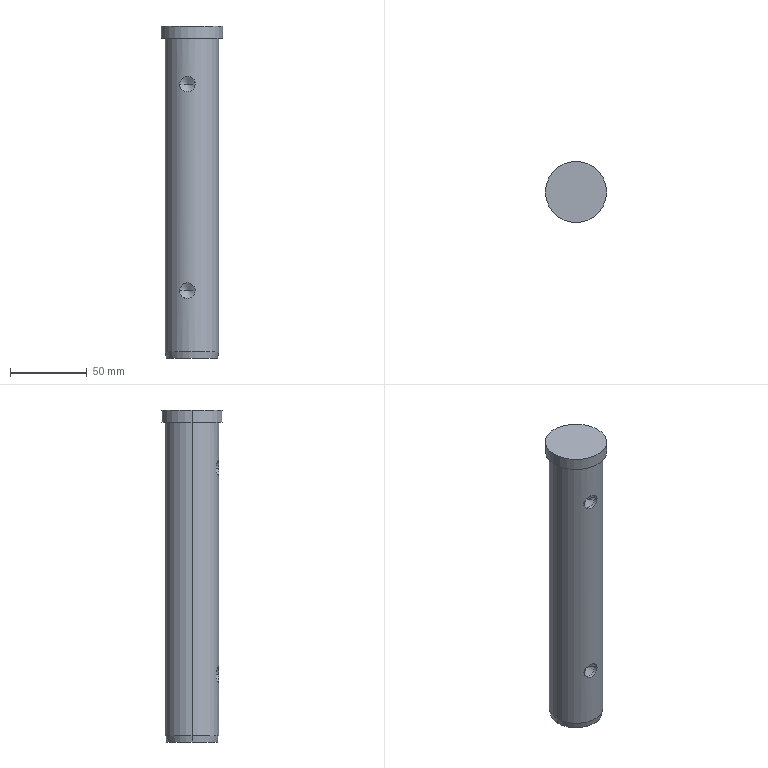Part | Creo | 1 solid | 17 faces | box 40 x 40 x 217 mm | volume 210497 mm3 | cylinder 8 | cone 6 | plane 3 | commonest cylinder face diameters 10.2 x4 35 x2 40 x2
STEP:
#1=CARTESIAN_POINT('',(0.,0.,0.));
#2=DIRECTION('',(0.,0.,1.));
#3=DIRECTION('',(1.,0.,0.));
#4=AXIS2_PLACEMENT_3D('',#1,#2,#3);
#5=CARTESIAN_POINT('',(-142.,-212.,112.5));
#6=VERTEX_POINT('',#5);
#7=CARTESIAN_POINT('',(-182.,-212.,112.5));
#8=VERTEX_POINT('',#7);
#9=CARTESIAN_POINT('',(-162.,-212.,112.5));
#10=DIRECTION('',(0.,0.,-1.));
#11=DIRECTION('',(1.,0.,0.));
#12=AXIS2_PLACEMENT_3D('',#9,#10,#11);
#13=CIRCLE('',#12,20.);
#14=EDGE_CURVE('',#6,#8,#13,.T.);
#15=ORIENTED_EDGE('',*,*,#14,.T.);
#16=CARTESIAN_POINT('',(-182.,-212.,120.5));
#17=VERTEX_POINT('',#16);
#18=CARTESIAN_POINT('',(-182.,-212.,112.5));
#19=DIRECTION('',(0.,0.,1.));
#20=VECTOR('',#19,8.);
#21=LINE('',#18,#20);
#22=EDGE_CURVE('',#8,#17,#21,.T.);
#23=ORIENTED_EDGE('',*,*,#22,.T.);
#24=CARTESIAN_POINT('',(-142.,-212.,120.5));
#25=VERTEX_POINT('',#24);
#26=CARTESIAN_POINT('',(-162.,-212.,120.5));
#27=DIRECTION('',(0.,0.,1.));
#28=DIRECTION('',(-1.,0.,0.));
#29=AXIS2_PLACEMENT_3D('',#26,#27,#28);
#30=CIRCLE('',#29,20.);
#31=EDGE_CURVE('',#17,#25,#30,.T.);
#32=ORIENTED_EDGE('',*,*,#31,.T.);
#33=CARTESIAN_POINT('',(-142.,-212.,112.5));
#34=DIRECTION('',(0.,0.,1.));
#35=VECTOR('',#34,8.);
#36=LINE('',#33,#35);
#37=EDGE_CURVE('',#6,#25,#36,.T.);
#38=ORIENTED_EDGE('',*,*,#37,.F.);
#39=EDGE_LOOP('',(#15,#23,#32,#38));
#40=FACE_OUTER_BOUND('',#39,.F.);
#41=CARTESIAN_POINT('',(-162.,-212.,112.5));
#42=DIRECTION('',(0.,0.,1.));
#43=DIRECTION('',(-1.,0.,0.));
#44=AXIS2_PLACEMENT_3D('',#41,#42,#43);
#45=CYLINDRICAL_SURFACE('',#44,20.);
#46=ADVANCED_FACE('',(#40),#45,.T.);
#47=ORIENTED_EDGE('',*,*,#14,.F.);
#48=CARTESIAN_POINT('',(-162.,-212.,112.5));
#49=DIRECTION('',(0.,0.,-1.));
#50=DIRECTION('',(-1.,0.,0.));
#51=AXIS2_PLACEMENT_3D('',#48,#49,#50);
#52=CIRCLE('',#51,20.);
#53=EDGE_CURVE('',#8,#6,#52,.T.);
#54=ORIENTED_EDGE('',*,*,#53,.F.);
#55=EDGE_LOOP('',(#47,#54));
#56=FACE_OUTER_BOUND('',#55,.F.);
#57=CARTESIAN_POINT('',(-179.5,-212.,112.5));
#58=VERTEX_POINT('',#57);
#59=CARTESIAN_POINT('',(-144.5,-212.,112.5));
#60=VERTEX_POINT('',#59);
#61=CARTESIAN_POINT('',(-162.,-212.,112.5));
#62=DIRECTION('',(0.,0.,1.));
#63=DIRECTION('',(-1.,0.,0.));
#64=AXIS2_PLACEMENT_3D('',#61,#62,#63);
#65=CIRCLE('',#64,17.5);
#66=EDGE_CURVE('',#58,#60,#65,.T.);
#67=ORIENTED_EDGE('',*,*,#66,.F.);
#68=CARTESIAN_POINT('',(-162.,-212.,112.5));
#69=DIRECTION('',(0.,0.,1.));
#70=DIRECTION('',(1.,0.,0.));
#71=AXIS2_PLACEMENT_3D('',#68,#69,#70);
#72=CIRCLE('',#71,17.5);
#73=EDGE_CURVE('',#60,#58,#72,.T.);
#74=ORIENTED_EDGE('',*,*,#73,.F.);
#75=EDGE_LOOP('',(#67,#74));
#76=FACE_BOUND('',#75,.F.);
#77=CARTESIAN_POINT('',(-162.,-212.,112.5));
#78=DIRECTION('',(0.,0.,1.));
#79=DIRECTION('',(-1.,0.,0.));
#80=AXIS2_PLACEMENT_3D('',#77,#78,#79);
#81=PLANE('',#80);
#82=ADVANCED_FACE('',(#56,#76),#81,.F.);
#83=CARTESIAN_POINT('',(-144.5,-212.,-92.5));
#84=VERTEX_POINT('',#83);
#85=CARTESIAN_POINT('',(-179.5,-212.,-92.5));
#86=VERTEX_POINT('',#85);
#87=CARTESIAN_POINT('',(-162.,-212.,-92.5));
#88=DIRECTION('',(0.,0.,-1.));
#89=DIRECTION('',(1.,0.,0.));
#90=AXIS2_PLACEMENT_3D('',#87,#88,#89);
#91=CIRCLE('',#90,17.5);
#92=EDGE_CURVE('',#84,#86,#91,.T.);
#93=ORIENTED_EDGE('',*,*,#92,.T.);
#94=CARTESIAN_POINT('',(-179.5,-212.,112.5));
#95=DIRECTION('',(0.,0.,-1.));
#96=VECTOR('',#95,205.);
#97=LINE('',#94,#96);
#98=EDGE_CURVE('',#58,#86,#97,.T.);
#99=ORIENTED_EDGE('',*,*,#98,.F.);
#100=ORIENTED_EDGE('',*,*,#66,.T.);
#101=CARTESIAN_POINT('',(-144.5,-212.,112.5));
#102=DIRECTION('',(0.,0.,-1.));
#103=VECTOR('',#102,205.);
#104=LINE('',#101,#103);
#105=EDGE_CURVE('',#60,#84,#104,.T.);
#106=ORIENTED_EDGE('',*,*,#105,.T.);
#107=EDGE_LOOP('',(#93,#99,#100,#106));
#108=FACE_OUTER_BOUND('',#107,.F.);
#109=CARTESIAN_POINT('',(-170.1,-227.513,82.5));
#110=VERTEX_POINT('',#109);
#111=CARTESIAN_POINT('',(-159.9,-229.374,82.5));
#112=VERTEX_POINT('',#111);
#113=CARTESIAN_POINT('',(-170.1,-227.513,82.5));
#114=CARTESIAN_POINT('',(-170.1,-227.513,82.927));
#115=CARTESIAN_POINT('',(-169.996,-227.567,83.761));
#116=CARTESIAN_POINT('',(-169.521,-227.806,84.981));
#117=CARTESIAN_POINT('',(-168.726,-228.167,86.072));
#118=CARTESIAN_POINT('',(-167.635,-228.584,86.939));
#119=CARTESIAN_POINT('',(-166.374,-228.962,87.472));
#120=CARTESIAN_POINT('',(-165.054,-229.249,87.656));
#121=CARTESIAN_POINT('',(-163.737,-229.43,87.501));
#122=CARTESIAN_POINT('',(-162.478,-229.507,87.001));
#123=CARTESIAN_POINT('',(-161.392,-229.498,86.189));
#124=CARTESIAN_POINT('',(-160.545,-229.444,85.108));
#125=CARTESIAN_POINT('',(-160.015,-229.388,83.829));
#126=CARTESIAN_POINT('',(-159.9,-229.374,82.953));
#127=CARTESIAN_POINT('',(-159.9,-229.374,82.5));
#128=B_SPLINE_CURVE_WITH_KNOTS('',3,(#113,#114,#115,#116,#117,#118,#119,#120,#121,#122,#123,#124,#125,#126,#127),.UNSPECIFIED.,.F.,.F.,(4,1,1,1,1,1,1,1,1,1,1,1,4),(0.,0.08333,0.1667,0.25,0.3333,0.4167,0.5,0.5833,0.6667,0.75,0.8333,0.9167,1.),.UNSPECIFIED.);
#129=EDGE_CURVE('',#110,#112,#128,.T.);
#130=ORIENTED_EDGE('',*,*,#129,.F.);
#131=CARTESIAN_POINT('',(-159.9,-229.374,82.5));
#132=CARTESIAN_POINT('',(-159.9,-229.374,82.038));
#133=CARTESIAN_POINT('',(-160.02,-229.389,81.149));
#134=CARTESIAN_POINT('',(-160.556,-229.445,79.875));
#135=CARTESIAN_POINT('',(-161.399,-229.499,78.805));
#136=CARTESIAN_POINT('',(-162.485,-229.507,77.995));
#137=CARTESIAN_POINT('',(-163.748,-229.429,77.496));
#138=CARTESIAN_POINT('',(-165.067,-229.247,77.344));
#139=CARTESIAN_POINT('',(-166.382,-228.96,77.53));
#140=CARTESIAN_POINT('',(-167.638,-228.583,78.063));
#141=CARTESIAN_POINT('',(-168.727,-228.166,78.93));
#142=CARTESIAN_POINT('',(-169.523,-227.805,80.022));
#143=CARTESIAN_POINT('',(-169.996,-227.567,81.241));
#144=CARTESIAN_POINT('',(-170.1,-227.513,82.073));
#145=CARTESIAN_POINT('',(-170.1,-227.513,82.5));
#146=B_SPLINE_CURVE_WITH_KNOTS('',3,(#131,#132,#133,#134,#135,#136,#137,#138,#139,#140,#141,#142,#143,#144,#145),.UNSPECIFIED.,.F.,.F.,(4,1,1,1,1,1,1,1,1,1,1,1,4),(0.,0.08333,0.1667,0.25,0.3333,0.4167,0.5,0.5833,0.6667,0.75,0.8333,0.9167,1.),.UNSPECIFIED.);
#147=EDGE_CURVE('',#112,#110,#146,.T.);
#148=ORIENTED_EDGE('',*,*,#147,.F.);
#149=EDGE_LOOP('',(#130,#148));
#150=FACE_BOUND('',#149,.F.);
#151=CARTESIAN_POINT('',(-170.1,-227.513,-52.5));
#152=VERTEX_POINT('',#151);
#153=CARTESIAN_POINT('',(-159.9,-229.374,-52.5));
#154=VERTEX_POINT('',#153);
#155=CARTESIAN_POINT('',(-170.1,-227.513,-52.5));
#156=CARTESIAN_POINT('',(-170.1,-227.513,-52.073));
#157=CARTESIAN_POINT('',(-169.996,-227.567,-51.239));
#158=CARTESIAN_POINT('',(-169.521,-227.806,-50.019));
#159=CARTESIAN_POINT('',(-168.726,-228.167,-48.928));
#160=CARTESIAN_POINT('',(-167.635,-228.584,-48.061));
#161=CARTESIAN_POINT('',(-166.374,-228.962,-47.528));
#162=CARTESIAN_POINT('',(-165.054,-229.249,-47.344));
#163=CARTESIAN_POINT('',(-163.737,-229.43,-47.499));
#164=CARTESIAN_POINT('',(-162.478,-229.507,-47.999));
#165=CARTESIAN_POINT('',(-161.392,-229.498,-48.811));
#166=CARTESIAN_POINT('',(-160.545,-229.444,-49.892));
#167=CARTESIAN_POINT('',(-160.015,-229.388,-51.171));
#168=CARTESIAN_POINT('',(-159.9,-229.374,-52.047));
#169=CARTESIAN_POINT('',(-159.9,-229.374,-52.5));
#170=B_SPLINE_CURVE_WITH_KNOTS('',3,(#155,#156,#157,#158,#159,#160,#161,#162,#163,#164,#165,#166,#167,#168,#169),.UNSPECIFIED.,.F.,.F.,(4,1,1,1,1,1,1,1,1,1,1,1,4),(0.,0.08333,0.1667,0.25,0.3333,0.4167,0.5,0.5833,0.6667,0.75,0.8333,0.9167,1.),.UNSPECIFIED.);
#171=EDGE_CURVE('',#152,#154,#170,.T.);
#172=ORIENTED_EDGE('',*,*,#171,.F.);
#173=CARTESIAN_POINT('',(-159.9,-229.374,-52.5));
#174=CARTESIAN_POINT('',(-159.9,-229.374,-52.962));
#175=CARTESIAN_POINT('',(-160.02,-229.389,-53.851));
#176=CARTESIAN_POINT('',(-160.556,-229.445,-55.125));
#177=CARTESIAN_POINT('',(-161.399,-229.499,-56.195));
#178=CARTESIAN_POINT('',(-162.485,-229.507,-57.005));
#179=CARTESIAN_POINT('',(-163.748,-229.429,-57.504));
#180=CARTESIAN_POINT('',(-165.067,-229.247,-57.656));
#181=CARTESIAN_POINT('',(-166.382,-228.96,-57.47));
#182=CARTESIAN_POINT('',(-167.638,-228.583,-56.937));
#183=CARTESIAN_POINT('',(-168.727,-228.166,-56.07));
#184=CARTESIAN_POINT('',(-169.523,-227.805,-54.978));
#185=CARTESIAN_POINT('',(-169.996,-227.567,-53.759));
#186=CARTESIAN_POINT('',(-170.1,-227.513,-52.927));
#187=CARTESIAN_POINT('',(-170.1,-227.513,-52.5));
#188=B_SPLINE_CURVE_WITH_KNOTS('',3,(#173,#174,#175,#176,#177,#178,#179,#180,#181,#182,#183,#184,#185,#186,#187),.UNSPECIFIED.,.F.,.F.,(4,1,1,1,1,1,1,1,1,1,1,1,4),(0.,0.08333,0.1667,0.25,0.3333,0.4167,0.5,0.5833,0.6667,0.75,0.8333,0.9167,1.),.UNSPECIFIED.);
#189=EDGE_CURVE('',#154,#152,#188,.T.);
#190=ORIENTED_EDGE('',*,*,#189,.F.);
#191=EDGE_LOOP('',(#172,#190));
#192=FACE_BOUND('',#191,.F.);
#193=CARTESIAN_POINT('',(-162.,-212.,112.5));
#194=DIRECTION('',(0.,0.,-1.));
#195=DIRECTION('',(1.,0.,0.));
#196=AXIS2_PLACEMENT_3D('',#193,#194,#195);
#197=CYLINDRICAL_SURFACE('',#196,17.5);
#198=ADVANCED_FACE('',(#108,#150,#192),#197,.T.);
#199=ORIENTED_EDGE('',*,*,#171,.T.);
#200=CARTESIAN_POINT('',(-159.9,-227.1,-52.5));
#201=VERTEX_POINT('',#200);
#202=CARTESIAN_POINT('',(-159.9,-227.1,-52.5));
#203=DIRECTION('',(-0.000000022,-1.,-0.0001831));
#204=VECTOR('',#203,2.274);
#205=LINE('',#202,#204);
#206=EDGE_CURVE('',#201,#154,#205,.T.);
#207=ORIENTED_EDGE('',*,*,#206,.F.);
#208=CARTESIAN_POINT('',(-170.1,-227.1,-52.5));
#209=VERTEX_POINT('',#208);
#210=CARTESIAN_POINT('',(-165.,-227.1,-52.5));
#211=DIRECTION('',(0.,-1.,0.));
#212=DIRECTION('',(1.,0.,0.));
#213=AXIS2_PLACEMENT_3D('',#210,#211,#212);
#214=CIRCLE('',#213,5.1);
#215=EDGE_CURVE('',#201,#209,#214,.T.);
#216=ORIENTED_EDGE('',*,*,#215,.T.);
#217=CARTESIAN_POINT('',(-170.1,-227.1,-52.5));
#218=DIRECTION('',(0.,-1.,0.));
#219=VECTOR('',#218,0.4126);
#220=LINE('',#217,#219);
#221=EDGE_CURVE('',#209,#152,#220,.T.);
#222=ORIENTED_EDGE('',*,*,#221,.T.);
#223=EDGE_LOOP('',(#199,#207,#216,#222));
#224=FACE_OUTER_BOUND('',#223,.F.);
#225=CARTESIAN_POINT('',(-165.,-300.,-52.5));
#226=DIRECTION('',(0.,-1.,0.));
#227=DIRECTION('',(-1.,0.,0.));
#228=AXIS2_PLACEMENT_3D('',#225,#226,#227);
#229=CYLINDRICAL_SURFACE('',#228,5.1);
#230=ADVANCED_FACE('',(#224),#229,.F.);
#231=ORIENTED_EDGE('',*,*,#189,.T.);
#232=ORIENTED_EDGE('',*,*,#221,.F.);
#233=CARTESIAN_POINT('',(-165.,-227.1,-52.5));
#234=DIRECTION('',(0.,-1.,0.));
#235=DIRECTION('',(-1.,0.,0.));
#236=AXIS2_PLACEMENT_3D('',#233,#234,#235);
#237=CIRCLE('',#236,5.1);
#238=EDGE_CURVE('',#209,#201,#237,.T.);
#239=ORIENTED_EDGE('',*,*,#238,.T.);
#240=ORIENTED_EDGE('',*,*,#206,.T.);
#241=EDGE_LOOP('',(#231,#232,#239,#240));
#242=FACE_OUTER_BOUND('',#241,.F.);
#243=CARTESIAN_POINT('',(-165.,-300.,-52.5));
#244=DIRECTION('',(0.,-1.,0.));
#245=DIRECTION('',(-1.,0.,0.));
#246=AXIS2_PLACEMENT_3D('',#243,#244,#245);
#247=CYLINDRICAL_SURFACE('',#246,5.1);
#248=ADVANCED_FACE('',(#242),#247,.F.);
#249=ORIENTED_EDGE('',*,*,#238,.F.);
#250=CARTESIAN_POINT('',(-165.,-224.036,-52.5));
#251=VERTEX_POINT('',#250);
#252=CARTESIAN_POINT('',(-165.,-224.036,-52.5));
#253=DIRECTION('',(-0.8572,-0.515,0.));
#254=VECTOR('',#253,5.95);
#255=LINE('',#252,#254);
#256=EDGE_CURVE('',#251,#209,#255,.T.);
#257=ORIENTED_EDGE('',*,*,#256,.F.);
#258=CARTESIAN_POINT('',(-165.,-224.036,-52.5));
#259=DIRECTION('',(0.8572,-0.515,0.));
#260=VECTOR('',#259,5.95);
#261=LINE('',#258,#260);
#262=EDGE_CURVE('',#251,#201,#261,.T.);
#263=ORIENTED_EDGE('',*,*,#262,.T.);
#264=EDGE_LOOP('',(#249,#257,#263));
#265=FACE_OUTER_BOUND('',#264,.F.);
#266=CARTESIAN_POINT('',(-165.,-225.637,-52.5));
#267=DIRECTION('',(0.,-1.,0.));
#268=DIRECTION('',(-1.,0.,0.));
#269=AXIS2_PLACEMENT_3D('',#266,#267,#268);
#270=CONICAL_SURFACE('',#269,2.665,59.);
#271=ADVANCED_FACE('',(#265),#270,.F.);
#272=ORIENTED_EDGE('',*,*,#215,.F.);
#273=ORIENTED_EDGE('',*,*,#262,.F.);
#274=ORIENTED_EDGE('',*,*,#256,.T.);
#275=EDGE_LOOP('',(#272,#273,#274));
#276=FACE_OUTER_BOUND('',#275,.F.);
#277=CARTESIAN_POINT('',(-165.,-225.637,-52.5));
#278=DIRECTION('',(0.,-1.,0.));
#279=DIRECTION('',(-1.,0.,0.));
#280=AXIS2_PLACEMENT_3D('',#277,#278,#279);
#281=CONICAL_SURFACE('',#280,2.665,59.);
#282=ADVANCED_FACE('',(#276),#281,.F.);
#283=ORIENTED_EDGE('',*,*,#129,.T.);
#284=CARTESIAN_POINT('',(-159.9,-227.1,82.5));
#285=VERTEX_POINT('',#284);
#286=CARTESIAN_POINT('',(-159.9,-227.1,82.5));
#287=DIRECTION('',(-0.000000022,-1.,-0.0001831));
#288=VECTOR('',#287,2.274);
#289=LINE('',#286,#288);
#290=EDGE_CURVE('',#285,#112,#289,.T.);
#291=ORIENTED_EDGE('',*,*,#290,.F.);
#292=CARTESIAN_POINT('',(-170.1,-227.1,82.5));
#293=VERTEX_POINT('',#292);
#294=CARTESIAN_POINT('',(-165.,-227.1,82.5));
#295=DIRECTION('',(0.,-1.,0.));
#296=DIRECTION('',(1.,0.,0.));
#297=AXIS2_PLACEMENT_3D('',#294,#295,#296);
#298=CIRCLE('',#297,5.1);
#299=EDGE_CURVE('',#285,#293,#298,.T.);
#300=ORIENTED_EDGE('',*,*,#299,.T.);
#301=CARTESIAN_POINT('',(-170.1,-227.1,82.5));
#302=DIRECTION('',(0.,-1.,0.));
#303=VECTOR('',#302,0.4126);
#304=LINE('',#301,#303);
#305=EDGE_CURVE('',#293,#110,#304,.T.);
#306=ORIENTED_EDGE('',*,*,#305,.T.);
#307=EDGE_LOOP('',(#283,#291,#300,#306));
#308=FACE_OUTER_BOUND('',#307,.F.);
#309=CARTESIAN_POINT('',(-165.,-300.,82.5));
#310=DIRECTION('',(0.,-1.,0.));
#311=DIRECTION('',(-1.,0.,0.));
#312=AXIS2_PLACEMENT_3D('',#309,#310,#311);
#313=CYLINDRICAL_SURFACE('',#312,5.1);
#314=ADVANCED_FACE('',(#308),#313,.F.);
#315=ORIENTED_EDGE('',*,*,#147,.T.);
#316=ORIENTED_EDGE('',*,*,#305,.F.);
#317=CARTESIAN_POINT('',(-165.,-227.1,82.5));
#318=DIRECTION('',(0.,-1.,0.));
#319=DIRECTION('',(-1.,0.,0.));
#320=AXIS2_PLACEMENT_3D('',#317,#318,#319);
#321=CIRCLE('',#320,5.1);
#322=EDGE_CURVE('',#293,#285,#321,.T.);
#323=ORIENTED_EDGE('',*,*,#322,.T.);
#324=ORIENTED_EDGE('',*,*,#290,.T.);
#325=EDGE_LOOP('',(#315,#316,#323,#324));
#326=FACE_OUTER_BOUND('',#325,.F.);
#327=CARTESIAN_POINT('',(-165.,-300.,82.5));
#328=DIRECTION('',(0.,-1.,0.));
#329=DIRECTION('',(-1.,0.,0.));
#330=AXIS2_PLACEMENT_3D('',#327,#328,#329);
#331=CYLINDRICAL_SURFACE('',#330,5.1);
#332=ADVANCED_FACE('',(#326),#331,.F.);
#333=ORIENTED_EDGE('',*,*,#322,.F.);
#334=CARTESIAN_POINT('',(-165.,-224.036,82.5));
#335=VERTEX_POINT('',#334);
#336=CARTESIAN_POINT('',(-165.,-224.036,82.5));
#337=DIRECTION('',(-0.8572,-0.515,0.));
#338=VECTOR('',#337,5.95);
#339=LINE('',#336,#338);
#340=EDGE_CURVE('',#335,#293,#339,.T.);
#341=ORIENTED_EDGE('',*,*,#340,.F.);
#342=CARTESIAN_POINT('',(-165.,-224.036,82.5));
#343=DIRECTION('',(0.8572,-0.515,0.));
#344=VECTOR('',#343,5.95);
#345=LINE('',#342,#344);
#346=EDGE_CURVE('',#335,#285,#345,.T.);
#347=ORIENTED_EDGE('',*,*,#346,.T.);
#348=EDGE_LOOP('',(#333,#341,#347));
#349=FACE_OUTER_BOUND('',#348,.F.);
#350=CARTESIAN_POINT('',(-165.,-225.637,82.5));
#351=DIRECTION('',(0.,-1.,0.));
#352=DIRECTION('',(-1.,0.,0.));
#353=AXIS2_PLACEMENT_3D('',#350,#351,#352);
#354=CONICAL_SURFACE('',#353,2.665,59.);
#355=ADVANCED_FACE('',(#349),#354,.F.);
#356=ORIENTED_EDGE('',*,*,#299,.F.);
#357=ORIENTED_EDGE('',*,*,#346,.F.);
#358=ORIENTED_EDGE('',*,*,#340,.T.);
#359=EDGE_LOOP('',(#356,#357,#358));
#360=FACE_OUTER_BOUND('',#359,.F.);
#361=CARTESIAN_POINT('',(-165.,-225.637,82.5));
#362=DIRECTION('',(0.,-1.,0.));
#363=DIRECTION('',(-1.,0.,0.));
#364=AXIS2_PLACEMENT_3D('',#361,#362,#363);
#365=CONICAL_SURFACE('',#364,2.665,59.);
#366=ADVANCED_FACE('',(#360),#365,.F.);
#367=ORIENTED_EDGE('',*,*,#92,.F.);
#368=CARTESIAN_POINT('',(-145.205,-212.,-96.5));
#369=VERTEX_POINT('',#368);
#370=CARTESIAN_POINT('',(-145.205,-212.,-96.5));
#371=DIRECTION('',(0.1736,0.,0.9848));
#372=VECTOR('',#371,4.062);
#373=LINE('',#370,#372);
#374=EDGE_CURVE('',#369,#84,#373,.T.);
#375=ORIENTED_EDGE('',*,*,#374,.F.);
#376=CARTESIAN_POINT('',(-178.795,-212.,-96.5));
#377=VERTEX_POINT('',#376);
#378=CARTESIAN_POINT('',(-162.,-212.,-96.5));
#379=DIRECTION('',(0.,0.,-1.));
#380=DIRECTION('',(1.,0.,0.));
#381=AXIS2_PLACEMENT_3D('',#378,#379,#380);
#382=CIRCLE('',#381,16.795);
#383=EDGE_CURVE('',#369,#377,#382,.T.);
#384=ORIENTED_EDGE('',*,*,#383,.T.);
#385=CARTESIAN_POINT('',(-178.795,-212.,-96.5));
#386=DIRECTION('',(-0.1736,0.,0.9848));
#387=VECTOR('',#386,4.062);
#388=LINE('',#385,#387);
#389=EDGE_CURVE('',#377,#86,#388,.T.);
#390=ORIENTED_EDGE('',*,*,#389,.T.);
#391=EDGE_LOOP('',(#367,#375,#384,#390));
#392=FACE_OUTER_BOUND('',#391,.F.);
#393=CARTESIAN_POINT('',(-162.,-212.,-94.5));
#394=DIRECTION('',(0.,0.,1.));
#395=DIRECTION('',(-1.,0.,0.));
#396=AXIS2_PLACEMENT_3D('',#393,#394,#395);
#397=CONICAL_SURFACE('',#396,17.147,10.);
#398=ADVANCED_FACE('',(#392),#397,.T.);
#399=CARTESIAN_POINT('',(-162.,-212.,-92.5));
#400=DIRECTION('',(0.,0.,-1.));
#401=DIRECTION('',(-1.,0.,0.));
#402=AXIS2_PLACEMENT_3D('',#399,#400,#401);
#403=CIRCLE('',#402,17.5);
#404=EDGE_CURVE('',#86,#84,#403,.T.);
#405=ORIENTED_EDGE('',*,*,#404,.F.);
#406=ORIENTED_EDGE('',*,*,#389,.F.);
#407=CARTESIAN_POINT('',(-162.,-212.,-96.5));
#408=DIRECTION('',(0.,0.,-1.));
#409=DIRECTION('',(-1.,0.,0.));
#410=AXIS2_PLACEMENT_3D('',#407,#408,#409);
#411=CIRCLE('',#410,16.795);
#412=EDGE_CURVE('',#377,#369,#411,.T.);
#413=ORIENTED_EDGE('',*,*,#412,.T.);
#414=ORIENTED_EDGE('',*,*,#374,.T.);
#415=EDGE_LOOP('',(#405,#406,#413,#414));
#416=FACE_OUTER_BOUND('',#415,.F.);
#417=CARTESIAN_POINT('',(-162.,-212.,-94.5));
#418=DIRECTION('',(0.,0.,1.));
#419=DIRECTION('',(-1.,0.,0.));
#420=AXIS2_PLACEMENT_3D('',#417,#418,#419);
#421=CONICAL_SURFACE('',#420,17.147,10.);
#422=ADVANCED_FACE('',(#416),#421,.T.);
#423=ORIENTED_EDGE('',*,*,#404,.T.);
#424=ORIENTED_EDGE('',*,*,#105,.F.);
#425=ORIENTED_EDGE('',*,*,#73,.T.);
#426=ORIENTED_EDGE('',*,*,#98,.T.);
#427=EDGE_LOOP('',(#423,#424,#425,#426));
#428=FACE_OUTER_BOUND('',#427,.F.);
#429=CARTESIAN_POINT('',(-162.,-212.,112.5));
#430=DIRECTION('',(0.,0.,-1.));
#431=DIRECTION('',(1.,0.,0.));
#432=AXIS2_PLACEMENT_3D('',#429,#430,#431);
#433=CYLINDRICAL_SURFACE('',#432,17.5);
#434=ADVANCED_FACE('',(#428),#433,.T.);
#435=ORIENTED_EDGE('',*,*,#412,.F.);
#436=ORIENTED_EDGE('',*,*,#383,.F.);
#437=EDGE_LOOP('',(#435,#436));
#438=FACE_OUTER_BOUND('',#437,.F.);
#439=CARTESIAN_POINT('',(-162.,-212.,-96.5));
#440=DIRECTION('',(0.,0.,-1.));
#441=DIRECTION('',(1.,0.,0.));
#442=AXIS2_PLACEMENT_3D('',#439,#440,#441);
#443=PLANE('',#442);
#444=ADVANCED_FACE('',(#438),#443,.T.);
#445=ORIENTED_EDGE('',*,*,#53,.T.);
#446=ORIENTED_EDGE('',*,*,#37,.T.);
#447=CARTESIAN_POINT('',(-162.,-212.,120.5));
#448=DIRECTION('',(0.,0.,1.));
#449=DIRECTION('',(1.,0.,0.));
#450=AXIS2_PLACEMENT_3D('',#447,#448,#449);
#451=CIRCLE('',#450,20.);
#452=EDGE_CURVE('',#25,#17,#451,.T.);
#453=ORIENTED_EDGE('',*,*,#452,.T.);
#454=ORIENTED_EDGE('',*,*,#22,.F.);
#455=EDGE_LOOP('',(#445,#446,#453,#454));
#456=FACE_OUTER_BOUND('',#455,.F.);
#457=CARTESIAN_POINT('',(-162.,-212.,112.5));
#458=DIRECTION('',(0.,0.,1.));
#459=DIRECTION('',(-1.,0.,0.));
#460=AXIS2_PLACEMENT_3D('',#457,#458,#459);
#461=CYLINDRICAL_SURFACE('',#460,20.);
#462=ADVANCED_FACE('',(#456),#461,.T.);
#463=ORIENTED_EDGE('',*,*,#452,.F.);
#464=ORIENTED_EDGE('',*,*,#31,.F.);
#465=EDGE_LOOP('',(#463,#464));
#466=FACE_OUTER_BOUND('',#465,.F.);
#467=CARTESIAN_POINT('',(-162.,-212.,120.5));
#468=DIRECTION('',(0.,0.,1.));
#469=DIRECTION('',(-1.,0.,0.));
#470=AXIS2_PLACEMENT_3D('',#467,#468,#469);
#471=PLANE('',#470);
#472=ADVANCED_FACE('',(#466),#471,.T.);
#473=CLOSED_SHELL('',(#46,#82,#198,#230,#248,#271,#282,#314,#332,#355,#366,#398,#422,#434,#444,#462,#472));
#474=MANIFOLD_SOLID_BREP('',#473);
#475=(LENGTH_UNIT()NAMED_UNIT(*)SI_UNIT(.MILLI.,.METRE.));
#476=UNCERTAINTY_MEASURE_WITH_UNIT(LENGTH_MEASURE(0.02243),#475,'','');
#477=(NAMED_UNIT(*)PLANE_ANGLE_UNIT()SI_UNIT($,.RADIAN.));
#478=PLANE_ANGLE_MEASURE_WITH_UNIT(PLANE_ANGLE_MEASURE(0.01745),#477);
#479=(CONVERSION_BASED_UNIT('DEGREE',#478)NAMED_UNIT(*)PLANE_ANGLE_UNIT());
#480=(NAMED_UNIT(*)SI_UNIT($,.STERADIAN.)SOLID_ANGLE_UNIT());
#481=(GEOMETRIC_REPRESENTATION_CONTEXT(3)GLOBAL_UNCERTAINTY_ASSIGNED_CONTEXT((#476))GLOBAL_UNIT_ASSIGNED_CONTEXT((#475,#479,#480))REPRESENTATION_CONTEXT('',''));
#482=ADVANCED_BREP_SHAPE_REPRESENTATION('',(#4,#474),#481);